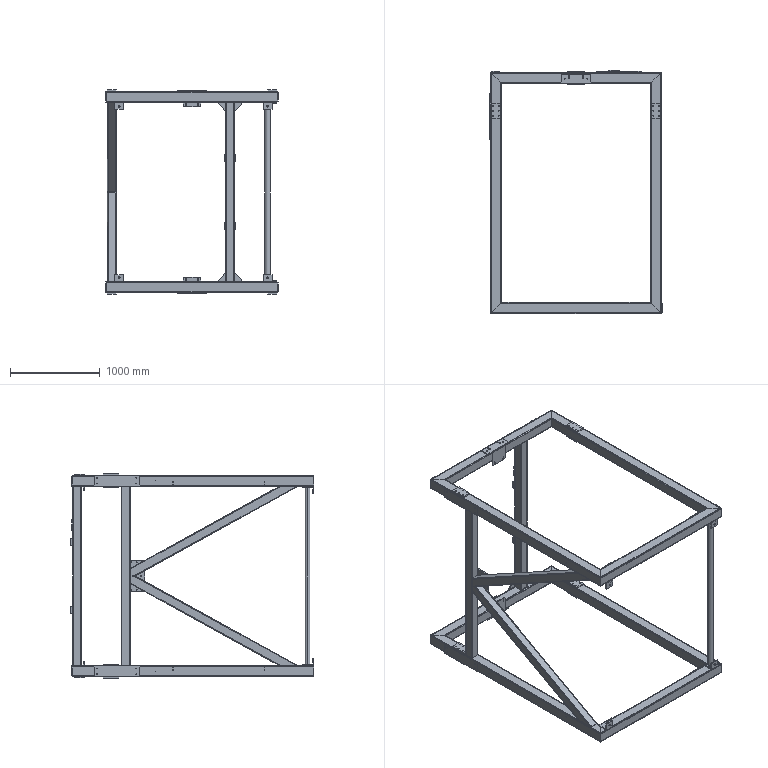Part | SolidWorks | features CompositeCurve 4 | 53 solids | 1129 faces | box 1920 x 2705 x 2270 mm | volume 52986318 mm3 | cylinder 742 | plane 387 | commonest cylinder face diameters 10.2 x202 15 x148 6.8 x68 5 x56 10 x48 20 x48